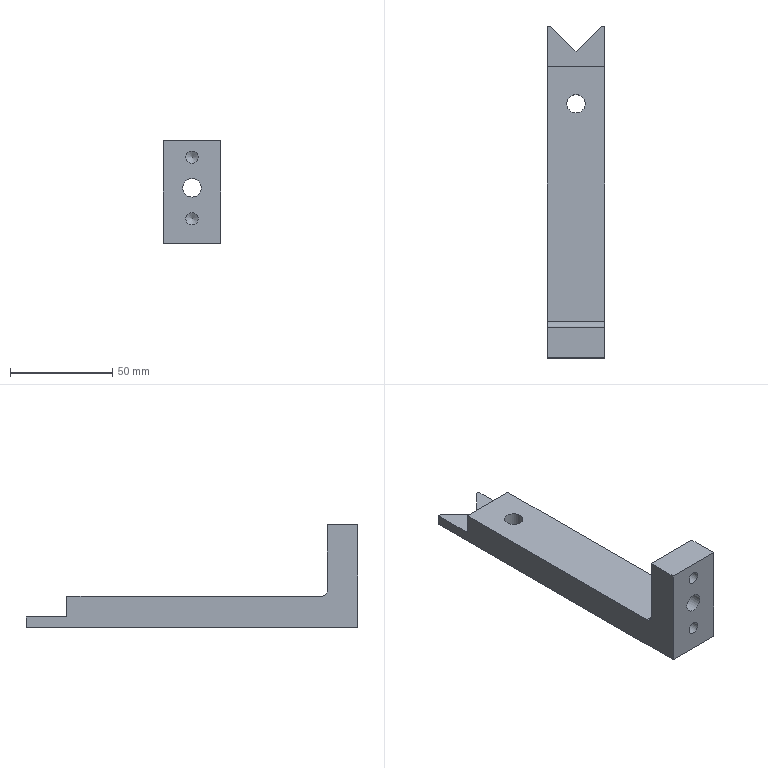Part | NX | features BREP 1 | 1 solid | 24 faces | box 28 x 162 x 50 mm | volume 73613 mm3 | plane 13 | cylinder 7 | cone 4 | commonest cylinder face diameters 6 x3 3.3 x2 9 x2
STEP:
#1=CARTESIAN_POINT('',(-4.5,43.,7.5));
#2=VERTEX_POINT('',#1);
#3=CARTESIAN_POINT('',(0.,43.,7.5));
#4=DIRECTION('',(0.,0.,-1.));
#5=DIRECTION('',(-1.,0.,0.));
#6=AXIS2_PLACEMENT_3D('',#3,#4,#5);
#7=CIRCLE('',#6,4.5);
#8=EDGE_CURVE('',#2,#2,#7,.T.);
#9=ORIENTED_EDGE('',*,*,#8,.T.);
#10=EDGE_LOOP('',(#9));
#11=FACE_BOUND('',#10,.T.);
#12=CARTESIAN_POINT('',(-14.,61.,7.5));
#13=VERTEX_POINT('',#12);
#14=CARTESIAN_POINT('',(-14.,-63.,7.5));
#15=VERTEX_POINT('',#14);
#16=CARTESIAN_POINT('',(-14.,-81.,7.5));
#17=DIRECTION('',(0.,-1.,0.));
#18=VECTOR('',#17,1000.);
#19=LINE('',#16,#18);
#20=EDGE_CURVE('',#13,#15,#19,.T.);
#21=ORIENTED_EDGE('',*,*,#20,.T.);
#22=CARTESIAN_POINT('',(14.,-63.,7.5));
#23=VERTEX_POINT('',#22);
#24=CARTESIAN_POINT('',(0.,-63.,7.5));
#25=DIRECTION('',(1.,0.,0.));
#26=VECTOR('',#25,1000.);
#27=LINE('',#24,#26);
#28=EDGE_CURVE('',#15,#23,#27,.T.);
#29=ORIENTED_EDGE('',*,*,#28,.T.);
#30=CARTESIAN_POINT('',(14.,61.,7.5));
#31=VERTEX_POINT('',#30);
#32=CARTESIAN_POINT('',(14.,-81.,7.5));
#33=DIRECTION('',(0.,1.,0.));
#34=VECTOR('',#33,1000.);
#35=LINE('',#32,#34);
#36=EDGE_CURVE('',#23,#31,#35,.T.);
#37=ORIENTED_EDGE('',*,*,#36,.T.);
#38=CARTESIAN_POINT('',(36.361,61.,7.5));
#39=DIRECTION('',(-1.,0.,0.));
#40=VECTOR('',#39,1000.);
#41=LINE('',#38,#40);
#42=EDGE_CURVE('',#31,#13,#41,.T.);
#43=ORIENTED_EDGE('',*,*,#42,.T.);
#44=EDGE_LOOP('',(#21,#29,#37,#43));
#45=FACE_BOUND('',#44,.T.);
#46=CARTESIAN_POINT('',(0.,0.,7.5));
#47=DIRECTION('',(0.,0.,-1.));
#48=DIRECTION('',(1.,0.,0.));
#49=AXIS2_PLACEMENT_3D('',#46,#47,#48);
#50=PLANE('',#49);
#51=ADVANCED_FACE('',(#11,#45),#50,.F.);
#52=CARTESIAN_POINT('',(-14.,81.,-2.5));
#53=VERTEX_POINT('',#52);
#54=CARTESIAN_POINT('',(-14.,81.,-7.5));
#55=VERTEX_POINT('',#54);
#56=CARTESIAN_POINT('',(-14.,81.,7.5));
#57=DIRECTION('',(0.,0.,-1.));
#58=VECTOR('',#57,1000.);
#59=LINE('',#56,#58);
#60=EDGE_CURVE('',#53,#55,#59,.T.);
#61=ORIENTED_EDGE('',*,*,#60,.F.);
#62=CARTESIAN_POINT('',(-12.5,81.,-2.5));
#63=VERTEX_POINT('',#62);
#64=CARTESIAN_POINT('',(36.361,81.,-2.5));
#65=DIRECTION('',(-1.,0.,0.));
#66=VECTOR('',#65,1000.);
#67=LINE('',#64,#66);
#68=EDGE_CURVE('',#63,#53,#67,.T.);
#69=ORIENTED_EDGE('',*,*,#68,.F.);
#70=CARTESIAN_POINT('',(-12.5,81.,-7.5));
#71=VERTEX_POINT('',#70);
#72=CARTESIAN_POINT('',(-12.5,81.,35.451));
#73=DIRECTION('',(0.,0.,-1.));
#74=VECTOR('',#73,1000.);
#75=LINE('',#72,#74);
#76=EDGE_CURVE('',#63,#71,#75,.T.);
#77=ORIENTED_EDGE('',*,*,#76,.T.);
#78=CARTESIAN_POINT('',(-14.,81.,-7.5));
#79=DIRECTION('',(-1.,0.,0.));
#80=VECTOR('',#79,1000.);
#81=LINE('',#78,#80);
#82=EDGE_CURVE('',#71,#55,#81,.T.);
#83=ORIENTED_EDGE('',*,*,#82,.T.);
#84=EDGE_LOOP('',(#61,#69,#77,#83));
#85=FACE_BOUND('',#84,.T.);
#86=CARTESIAN_POINT('',(-14.,81.,7.5));
#87=DIRECTION('',(0.,-1.,0.));
#88=DIRECTION('',(0.,0.,1.));
#89=AXIS2_PLACEMENT_3D('',#86,#87,#88);
#90=PLANE('',#89);
#91=ADVANCED_FACE('',(#85),#90,.F.);
#92=CARTESIAN_POINT('',(14.,61.,-2.5));
#93=VERTEX_POINT('',#92);
#94=CARTESIAN_POINT('',(14.,81.,-2.5));
#95=VERTEX_POINT('',#94);
#96=CARTESIAN_POINT('',(14.,61.,-2.5));
#97=DIRECTION('',(0.,1.,0.));
#98=VECTOR('',#97,1000.);
#99=LINE('',#96,#98);
#100=EDGE_CURVE('',#93,#95,#99,.T.);
#101=ORIENTED_EDGE('',*,*,#100,.F.);
#102=CARTESIAN_POINT('',(14.,61.,7.5));
#103=DIRECTION('',(0.,0.,-1.));
#104=VECTOR('',#103,1000.);
#105=LINE('',#102,#104);
#106=EDGE_CURVE('',#31,#93,#105,.T.);
#107=ORIENTED_EDGE('',*,*,#106,.F.);
#108=ORIENTED_EDGE('',*,*,#36,.F.);
#109=CARTESIAN_POINT('',(14.,-66.,10.5));
#110=VERTEX_POINT('',#109);
#111=CARTESIAN_POINT('',(14.,-63.,10.5));
#112=DIRECTION('',(-1.,0.,0.));
#113=DIRECTION('',(0.,0.,1.));
#114=AXIS2_PLACEMENT_3D('',#111,#112,#113);
#115=CIRCLE('',#114,3.);
#116=EDGE_CURVE('',#23,#110,#115,.T.);
#117=ORIENTED_EDGE('',*,*,#116,.T.);
#118=CARTESIAN_POINT('',(14.,-66.,42.5));
#119=VERTEX_POINT('',#118);
#120=CARTESIAN_POINT('',(14.,-66.,7.5));
#121=DIRECTION('',(0.,0.,1.));
#122=VECTOR('',#121,1000.);
#123=LINE('',#120,#122);
#124=EDGE_CURVE('',#110,#119,#123,.T.);
#125=ORIENTED_EDGE('',*,*,#124,.T.);
#126=CARTESIAN_POINT('',(14.,-81.,42.5));
#127=VERTEX_POINT('',#126);
#128=CARTESIAN_POINT('',(14.,-81.,42.5));
#129=DIRECTION('',(0.,-1.,0.));
#130=VECTOR('',#129,1000.);
#131=LINE('',#128,#130);
#132=EDGE_CURVE('',#119,#127,#131,.T.);
#133=ORIENTED_EDGE('',*,*,#132,.T.);
#134=CARTESIAN_POINT('',(14.,-81.,-7.5));
#135=VERTEX_POINT('',#134);
#136=CARTESIAN_POINT('',(14.,-81.,7.5));
#137=DIRECTION('',(0.,0.,-1.));
#138=VECTOR('',#137,1000.);
#139=LINE('',#136,#138);
#140=EDGE_CURVE('',#127,#135,#139,.T.);
#141=ORIENTED_EDGE('',*,*,#140,.T.);
#142=CARTESIAN_POINT('',(14.,81.,-7.5));
#143=VERTEX_POINT('',#142);
#144=CARTESIAN_POINT('',(14.,-81.,-7.5));
#145=DIRECTION('',(0.,1.,0.));
#146=VECTOR('',#145,1000.);
#147=LINE('',#144,#146);
#148=EDGE_CURVE('',#135,#143,#147,.T.);
#149=ORIENTED_EDGE('',*,*,#148,.T.);
#150=CARTESIAN_POINT('',(14.,81.,7.5));
#151=DIRECTION('',(0.,0.,-1.));
#152=VECTOR('',#151,1000.);
#153=LINE('',#150,#152);
#154=EDGE_CURVE('',#95,#143,#153,.T.);
#155=ORIENTED_EDGE('',*,*,#154,.F.);
#156=EDGE_LOOP('',(#101,#107,#108,#117,#125,#133,#141,#149,#155));
#157=FACE_BOUND('',#156,.T.);
#158=CARTESIAN_POINT('',(14.,-81.,7.5));
#159=DIRECTION('',(-1.,0.,0.));
#160=DIRECTION('',(0.,0.,-1.));
#161=AXIS2_PLACEMENT_3D('',#158,#159,#160);
#162=PLANE('',#161);
#163=ADVANCED_FACE('',(#157),#162,.F.);
#164=CARTESIAN_POINT('',(12.5,81.,-2.5));
#165=VERTEX_POINT('',#164);
#166=CARTESIAN_POINT('',(12.5,81.,-7.5));
#167=VERTEX_POINT('',#166);
#168=CARTESIAN_POINT('',(12.5,81.,35.451));
#169=DIRECTION('',(0.,0.,-1.));
#170=VECTOR('',#169,1000.);
#171=LINE('',#168,#170);
#172=EDGE_CURVE('',#165,#167,#171,.T.);
#173=ORIENTED_EDGE('',*,*,#172,.F.);
#174=CARTESIAN_POINT('',(36.361,81.,-2.5));
#175=DIRECTION('',(-1.,0.,0.));
#176=VECTOR('',#175,1000.);
#177=LINE('',#174,#176);
#178=EDGE_CURVE('',#95,#165,#177,.T.);
#179=ORIENTED_EDGE('',*,*,#178,.F.);
#180=ORIENTED_EDGE('',*,*,#154,.T.);
#181=CARTESIAN_POINT('',(-14.,81.,-7.5));
#182=DIRECTION('',(-1.,0.,0.));
#183=VECTOR('',#182,1000.);
#184=LINE('',#181,#183);
#185=EDGE_CURVE('',#143,#167,#184,.T.);
#186=ORIENTED_EDGE('',*,*,#185,.T.);
#187=EDGE_LOOP('',(#173,#179,#180,#186));
#188=FACE_BOUND('',#187,.T.);
#189=CARTESIAN_POINT('',(-14.,81.,7.5));
#190=DIRECTION('',(0.,-1.,0.));
#191=DIRECTION('',(0.,0.,1.));
#192=AXIS2_PLACEMENT_3D('',#189,#190,#191);
#193=PLANE('',#192);
#194=ADVANCED_FACE('',(#188),#193,.F.);
#195=ORIENTED_EDGE('',*,*,#20,.F.);
#196=CARTESIAN_POINT('',(-14.,61.,-2.5));
#197=VERTEX_POINT('',#196);
#198=CARTESIAN_POINT('',(-14.,61.,7.5));
#199=DIRECTION('',(0.,0.,1.));
#200=VECTOR('',#199,1000.);
#201=LINE('',#198,#200);
#202=EDGE_CURVE('',#197,#13,#201,.T.);
#203=ORIENTED_EDGE('',*,*,#202,.F.);
#204=CARTESIAN_POINT('',(-14.,61.,-2.5));
#205=DIRECTION('',(0.,-1.,0.));
#206=VECTOR('',#205,1000.);
#207=LINE('',#204,#206);
#208=EDGE_CURVE('',#53,#197,#207,.T.);
#209=ORIENTED_EDGE('',*,*,#208,.F.);
#210=ORIENTED_EDGE('',*,*,#60,.T.);
#211=CARTESIAN_POINT('',(-14.,-81.,-7.5));
#212=VERTEX_POINT('',#211);
#213=CARTESIAN_POINT('',(-14.,-81.,-7.5));
#214=DIRECTION('',(0.,-1.,0.));
#215=VECTOR('',#214,1000.);
#216=LINE('',#213,#215);
#217=EDGE_CURVE('',#55,#212,#216,.T.);
#218=ORIENTED_EDGE('',*,*,#217,.T.);
#219=CARTESIAN_POINT('',(-14.,-81.,42.5));
#220=VERTEX_POINT('',#219);
#221=CARTESIAN_POINT('',(-14.,-81.,7.5));
#222=DIRECTION('',(0.,0.,-1.));
#223=VECTOR('',#222,1000.);
#224=LINE('',#221,#223);
#225=EDGE_CURVE('',#220,#212,#224,.T.);
#226=ORIENTED_EDGE('',*,*,#225,.F.);
#227=CARTESIAN_POINT('',(-14.,-66.,42.5));
#228=VERTEX_POINT('',#227);
#229=CARTESIAN_POINT('',(-14.,-81.,42.5));
#230=DIRECTION('',(0.,1.,0.));
#231=VECTOR('',#230,1000.);
#232=LINE('',#229,#231);
#233=EDGE_CURVE('',#220,#228,#232,.T.);
#234=ORIENTED_EDGE('',*,*,#233,.T.);
#235=CARTESIAN_POINT('',(-14.,-66.,10.5));
#236=VERTEX_POINT('',#235);
#237=CARTESIAN_POINT('',(-14.,-66.,7.5));
#238=DIRECTION('',(0.,0.,-1.));
#239=VECTOR('',#238,1000.);
#240=LINE('',#237,#239);
#241=EDGE_CURVE('',#228,#236,#240,.T.);
#242=ORIENTED_EDGE('',*,*,#241,.T.);
#243=CARTESIAN_POINT('',(-14.,-63.,10.5));
#244=DIRECTION('',(1.,0.,0.));
#245=DIRECTION('',(0.,0.,-1.));
#246=AXIS2_PLACEMENT_3D('',#243,#244,#245);
#247=CIRCLE('',#246,3.);
#248=EDGE_CURVE('',#236,#15,#247,.T.);
#249=ORIENTED_EDGE('',*,*,#248,.T.);
#250=EDGE_LOOP('',(#195,#203,#209,#210,#218,#226,#234,#242,#249));
#251=FACE_BOUND('',#250,.T.);
#252=CARTESIAN_POINT('',(-14.,-81.,7.5));
#253=DIRECTION('',(1.,0.,0.));
#254=DIRECTION('',(0.,0.,1.));
#255=AXIS2_PLACEMENT_3D('',#252,#253,#254);
#256=PLANE('',#255);
#257=ADVANCED_FACE('',(#251),#256,.F.);
#258=CARTESIAN_POINT('',(0.,-81.,24.));
#259=VERTEX_POINT('',#258);
#260=CARTESIAN_POINT('',(0.,-81.,19.5));
#261=DIRECTION('',(0.,1.,0.));
#262=DIRECTION('',(0.,0.,1.));
#263=AXIS2_PLACEMENT_3D('',#260,#261,#262);
#264=CIRCLE('',#263,4.5);
#265=EDGE_CURVE('',#259,#259,#264,.T.);
#266=ORIENTED_EDGE('',*,*,#265,.T.);
#267=EDGE_LOOP('',(#266));
#268=FACE_BOUND('',#267,.T.);
#269=CARTESIAN_POINT('',(0.,-81.,31.5));
#270=VERTEX_POINT('',#269);
#271=CARTESIAN_POINT('',(0.,-81.,34.5));
#272=DIRECTION('',(0.,-1.,0.));
#273=DIRECTION('',(0.,0.,-1.));
#274=AXIS2_PLACEMENT_3D('',#271,#272,#273);
#275=CIRCLE('',#274,3.);
#276=EDGE_CURVE('',#270,#270,#275,.T.);
#277=ORIENTED_EDGE('',*,*,#276,.F.);
#278=EDGE_LOOP('',(#277));
#279=FACE_BOUND('',#278,.T.);
#280=CARTESIAN_POINT('',(0.,-81.,1.5));
#281=VERTEX_POINT('',#280);
#282=CARTESIAN_POINT('',(0.,-81.,4.5));
#283=DIRECTION('',(0.,-1.,0.));
#284=DIRECTION('',(0.,0.,-1.));
#285=AXIS2_PLACEMENT_3D('',#282,#283,#284);
#286=CIRCLE('',#285,3.);
#287=EDGE_CURVE('',#281,#281,#286,.T.);
#288=ORIENTED_EDGE('',*,*,#287,.F.);
#289=EDGE_LOOP('',(#288));
#290=FACE_BOUND('',#289,.T.);
#291=CARTESIAN_POINT('',(-14.,-81.,-7.5));
#292=DIRECTION('',(1.,0.,0.));
#293=VECTOR('',#292,1000.);
#294=LINE('',#291,#293);
#295=EDGE_CURVE('',#212,#135,#294,.T.);
#296=ORIENTED_EDGE('',*,*,#295,.T.);
#297=ORIENTED_EDGE('',*,*,#140,.F.);
#298=CARTESIAN_POINT('',(52.079,-81.,42.5));
#299=DIRECTION('',(-1.,0.,0.));
#300=VECTOR('',#299,1000.);
#301=LINE('',#298,#300);
#302=EDGE_CURVE('',#127,#220,#301,.T.);
#303=ORIENTED_EDGE('',*,*,#302,.T.);
#304=ORIENTED_EDGE('',*,*,#225,.T.);
#305=EDGE_LOOP('',(#296,#297,#303,#304));
#306=FACE_BOUND('',#305,.T.);
#307=CARTESIAN_POINT('',(-14.,-81.,7.5));
#308=DIRECTION('',(0.,1.,0.));
#309=DIRECTION('',(0.,0.,-1.));
#310=AXIS2_PLACEMENT_3D('',#307,#308,#309);
#311=PLANE('',#310);
#312=ADVANCED_FACE('',(#268,#279,#290,#306),#311,.F.);
#313=CARTESIAN_POINT('',(8.35,36.881,-7.5));
#314=VERTEX_POINT('',#313);
#315=CARTESIAN_POINT('',(10.,36.881,-7.5));
#316=DIRECTION('',(0.,0.,-1.));
#317=DIRECTION('',(-1.,0.,0.));
#318=AXIS2_PLACEMENT_3D('',#315,#316,#317);
#319=CIRCLE('',#318,1.65);
#320=EDGE_CURVE('',#314,#314,#319,.T.);
#321=ORIENTED_EDGE('',*,*,#320,.F.);
#322=EDGE_LOOP('',(#321));
#323=FACE_BOUND('',#322,.T.);
#324=CARTESIAN_POINT('',(-11.65,36.881,-7.5));
#325=VERTEX_POINT('',#324);
#326=CARTESIAN_POINT('',(-10.,36.881,-7.5));
#327=DIRECTION('',(0.,0.,-1.));
#328=DIRECTION('',(-1.,0.,0.));
#329=AXIS2_PLACEMENT_3D('',#326,#327,#328);
#330=CIRCLE('',#329,1.65);
#331=EDGE_CURVE('',#325,#325,#330,.T.);
#332=ORIENTED_EDGE('',*,*,#331,.F.);
#333=EDGE_LOOP('',(#332));
#334=FACE_BOUND('',#333,.T.);
#335=CARTESIAN_POINT('',(-4.5,43.,-7.5));
#336=VERTEX_POINT('',#335);
#337=CARTESIAN_POINT('',(0.,43.,-7.5));
#338=DIRECTION('',(0.,0.,-1.));
#339=DIRECTION('',(-1.,0.,0.));
#340=AXIS2_PLACEMENT_3D('',#337,#338,#339);
#341=CIRCLE('',#340,4.5);
#342=EDGE_CURVE('',#336,#336,#341,.T.);
#343=ORIENTED_EDGE('',*,*,#342,.F.);
#344=EDGE_LOOP('',(#343));
#345=FACE_BOUND('',#344,.T.);
#346=CARTESIAN_POINT('',(0.,68.5,-7.5));
#347=VERTEX_POINT('',#346);
#348=CARTESIAN_POINT('',(0.,68.5,-7.5));
#349=DIRECTION('',(-0.7071,0.7071,0.));
#350=VECTOR('',#349,1000.);
#351=LINE('',#348,#350);
#352=EDGE_CURVE('',#347,#71,#351,.T.);
#353=ORIENTED_EDGE('',*,*,#352,.F.);
#354=CARTESIAN_POINT('',(12.5,81.,-7.5));
#355=DIRECTION('',(-0.7071,-0.7071,0.));
#356=VECTOR('',#355,1000.);
#357=LINE('',#354,#356);
#358=EDGE_CURVE('',#167,#347,#357,.T.);
#359=ORIENTED_EDGE('',*,*,#358,.F.);
#360=ORIENTED_EDGE('',*,*,#185,.F.);
#361=ORIENTED_EDGE('',*,*,#148,.F.);
#362=ORIENTED_EDGE('',*,*,#295,.F.);
#363=ORIENTED_EDGE('',*,*,#217,.F.);
#364=ORIENTED_EDGE('',*,*,#82,.F.);
#365=EDGE_LOOP('',(#353,#359,#360,#361,#362,#363,#364));
#366=FACE_BOUND('',#365,.T.);
#367=CARTESIAN_POINT('',(0.,0.,-7.5));
#368=DIRECTION('',(0.,0.,-1.));
#369=DIRECTION('',(1.,0.,0.));
#370=AXIS2_PLACEMENT_3D('',#367,#368,#369);
#371=PLANE('',#370);
#372=ADVANCED_FACE('',(#323,#334,#345,#366),#371,.T.);
#373=ORIENTED_EDGE('',*,*,#76,.F.);
#374=CARTESIAN_POINT('',(0.,68.5,-2.5));
#375=VERTEX_POINT('',#374);
#376=CARTESIAN_POINT('',(0.,68.5,-2.5));
#377=DIRECTION('',(0.7071,-0.7071,0.));
#378=VECTOR('',#377,1000.);
#379=LINE('',#376,#378);
#380=EDGE_CURVE('',#63,#375,#379,.T.);
#381=ORIENTED_EDGE('',*,*,#380,.T.);
#382=CARTESIAN_POINT('',(0.,68.5,35.451));
#383=DIRECTION('',(0.,0.,-1.));
#384=VECTOR('',#383,1000.);
#385=LINE('',#382,#384);
#386=EDGE_CURVE('',#375,#347,#385,.T.);
#387=ORIENTED_EDGE('',*,*,#386,.T.);
#388=ORIENTED_EDGE('',*,*,#352,.T.);
#389=EDGE_LOOP('',(#373,#381,#387,#388));
#390=FACE_BOUND('',#389,.T.);
#391=CARTESIAN_POINT('',(0.,68.5,35.451));
#392=DIRECTION('',(-0.7071,-0.7071,0.));
#393=DIRECTION('',(-0.7071,0.7071,0.));
#394=AXIS2_PLACEMENT_3D('',#391,#392,#393);
#395=PLANE('',#394);
#396=ADVANCED_FACE('',(#390),#395,.F.);
#397=ORIENTED_EDGE('',*,*,#386,.F.);
#398=CARTESIAN_POINT('',(12.5,81.,-2.5));
#399=DIRECTION('',(0.7071,0.7071,0.));
#400=VECTOR('',#399,1000.);
#401=LINE('',#398,#400);
#402=EDGE_CURVE('',#375,#165,#401,.T.);
#403=ORIENTED_EDGE('',*,*,#402,.T.);
#404=ORIENTED_EDGE('',*,*,#172,.T.);
#405=ORIENTED_EDGE('',*,*,#358,.T.);
#406=EDGE_LOOP('',(#397,#403,#404,#405));
#407=FACE_BOUND('',#406,.T.);
#408=CARTESIAN_POINT('',(12.5,81.,35.451));
#409=DIRECTION('',(0.7071,-0.7071,0.));
#410=DIRECTION('',(-0.7071,-0.7071,0.));
#411=AXIS2_PLACEMENT_3D('',#408,#409,#410);
#412=PLANE('',#411);
#413=ADVANCED_FACE('',(#407),#412,.F.);
#414=ORIENTED_EDGE('',*,*,#68,.T.);
#415=ORIENTED_EDGE('',*,*,#208,.T.);
#416=CARTESIAN_POINT('',(36.361,61.,-2.5));
#417=DIRECTION('',(-1.,0.,0.));
#418=VECTOR('',#417,1000.);
#419=LINE('',#416,#418);
#420=EDGE_CURVE('',#93,#197,#419,.T.);
#421=ORIENTED_EDGE('',*,*,#420,.F.);
#422=ORIENTED_EDGE('',*,*,#100,.T.);
#423=ORIENTED_EDGE('',*,*,#178,.T.);
#424=ORIENTED_EDGE('',*,*,#402,.F.);
#425=ORIENTED_EDGE('',*,*,#380,.F.);
#426=EDGE_LOOP('',(#414,#415,#421,#422,#423,#424,#425));
#427=FACE_BOUND('',#426,.T.);
#428=CARTESIAN_POINT('',(36.361,61.,-2.5));
#429=DIRECTION('',(0.,0.,-1.));
#430=DIRECTION('',(0.,-1.,0.));
#431=AXIS2_PLACEMENT_3D('',#428,#429,#430);
#432=PLANE('',#431);
#433=ADVANCED_FACE('',(#427),#432,.F.);
#434=ORIENTED_EDGE('',*,*,#106,.T.);
#435=ORIENTED_EDGE('',*,*,#420,.T.);
#436=ORIENTED_EDGE('',*,*,#202,.T.);
#437=ORIENTED_EDGE('',*,*,#42,.F.);
#438=EDGE_LOOP('',(#434,#435,#436,#437));
#439=FACE_BOUND('',#438,.T.);
#440=CARTESIAN_POINT('',(36.361,61.,7.5));
#441=DIRECTION('',(0.,-1.,0.));
#442=DIRECTION('',(0.,0.,1.));
#443=AXIS2_PLACEMENT_3D('',#440,#441,#442);
#444=PLANE('',#443);
#445=ADVANCED_FACE('',(#439),#444,.F.);
#446=CARTESIAN_POINT('',(0.,-66.,24.));
#447=VERTEX_POINT('',#446);
#448=CARTESIAN_POINT('',(0.,-66.,19.5));
#449=DIRECTION('',(0.,1.,0.));
#450=DIRECTION('',(0.,0.,1.));
#451=AXIS2_PLACEMENT_3D('',#448,#449,#450);
#452=CIRCLE('',#451,4.5);
#453=EDGE_CURVE('',#447,#447,#452,.T.);
#454=ORIENTED_EDGE('',*,*,#453,.F.);
#455=EDGE_LOOP('',(#454));
#456=FACE_BOUND('',#455,.T.);
#457=ORIENTED_EDGE('',*,*,#124,.F.);
#458=CARTESIAN_POINT('',(52.079,-66.,10.5));
#459=DIRECTION('',(-1.,0.,0.));
#460=VECTOR('',#459,1000.);
#461=LINE('',#458,#460);
#462=EDGE_CURVE('',#110,#236,#461,.T.);
#463=ORIENTED_EDGE('',*,*,#462,.T.);
#464=ORIENTED_EDGE('',*,*,#241,.F.);
#465=CARTESIAN_POINT('',(52.079,-66.,42.5));
#466=DIRECTION('',(-1.,0.,0.));
#467=VECTOR('',#466,1000.);
#468=LINE('',#465,#467);
#469=EDGE_CURVE('',#119,#228,#468,.T.);
#470=ORIENTED_EDGE('',*,*,#469,.F.);
#471=EDGE_LOOP('',(#457,#463,#464,#470));
#472=FACE_BOUND('',#471,.T.);
#473=CARTESIAN_POINT('',(52.079,-66.,7.5));
#474=DIRECTION('',(0.,1.,0.));
#475=DIRECTION('',(0.,0.,-1.));
#476=AXIS2_PLACEMENT_3D('',#473,#474,#475);
#477=PLANE('',#476);
#478=ADVANCED_FACE('',(#456,#472),#477,.T.);
#479=ORIENTED_EDGE('',*,*,#132,.F.);
#480=ORIENTED_EDGE('',*,*,#469,.T.);
#481=ORIENTED_EDGE('',*,*,#233,.F.);
#482=ORIENTED_EDGE('',*,*,#302,.F.);
#483=EDGE_LOOP('',(#479,#480,#481,#482));
#484=FACE_BOUND('',#483,.T.);
#485=CARTESIAN_POINT('',(52.079,-81.,42.5));
#486=DIRECTION('',(0.,0.,1.));
#487=DIRECTION('',(-1.,0.,0.));
#488=AXIS2_PLACEMENT_3D('',#485,#486,#487);
#489=PLANE('',#488);
#490=ADVANCED_FACE('',(#484),#489,.T.);
#491=CARTESIAN_POINT('',(0.,-67.197,4.5));
#492=VERTEX_POINT('',#491);
#493=VERTEX_LOOP('',#492);
#494=FACE_BOUND('',#493,.T.);
#495=CARTESIAN_POINT('',(0.,-69.,1.5));
#496=VERTEX_POINT('',#495);
#497=CARTESIAN_POINT('',(0.,-69.,4.5));
#498=DIRECTION('',(0.,-1.,0.));
#499=DIRECTION('',(0.,0.,-1.));
#500=AXIS2_PLACEMENT_3D('',#497,#498,#499);
#501=CIRCLE('',#500,3.);
#502=EDGE_CURVE('',#496,#496,#501,.T.);
#503=ORIENTED_EDGE('',*,*,#502,.T.);
#504=EDGE_LOOP('',(#503));
#505=FACE_BOUND('',#504,.T.);
#506=CARTESIAN_POINT('',(0.,-69.,4.5));
#507=DIRECTION('',(0.,-1.,0.));
#508=DIRECTION('',(0.,0.,1.));
#509=AXIS2_PLACEMENT_3D('',#506,#507,#508);
#510=CONICAL_SURFACE('',#509,3.,1.03);
#511=ADVANCED_FACE('',(#494,#505),#510,.F.);
#512=ORIENTED_EDGE('',*,*,#502,.F.);
#513=EDGE_LOOP('',(#512));
#514=FACE_BOUND('',#513,.T.);
#515=ORIENTED_EDGE('',*,*,#287,.T.);
#516=EDGE_LOOP('',(#515));
#517=FACE_BOUND('',#516,.T.);
#518=CARTESIAN_POINT('',(0.,-81.,4.5));
#519=DIRECTION('',(0.,-1.,0.));
#520=DIRECTION('',(0.,0.,1.));
#521=AXIS2_PLACEMENT_3D('',#518,#519,#520);
#522=CYLINDRICAL_SURFACE('',#521,3.);
#523=ADVANCED_FACE('',(#514,#517),#522,.F.);
#524=CARTESIAN_POINT('',(0.,-67.197,34.5));
#525=VERTEX_POINT('',#524);
#526=VERTEX_LOOP('',#525);
#527=FACE_BOUND('',#526,.T.);
#528=CARTESIAN_POINT('',(0.,-69.,31.5));
#529=VERTEX_POINT('',#528);
#530=CARTESIAN_POINT('',(0.,-69.,34.5));
#531=DIRECTION('',(0.,-1.,0.));
#532=DIRECTION('',(0.,0.,-1.));
#533=AXIS2_PLACEMENT_3D('',#530,#531,#532);
#534=CIRCLE('',#533,3.);
#535=EDGE_CURVE('',#529,#529,#534,.T.);
#536=ORIENTED_EDGE('',*,*,#535,.T.);
#537=EDGE_LOOP('',(#536));
#538=FACE_BOUND('',#537,.T.);
#539=CARTESIAN_POINT('',(0.,-69.,34.5));
#540=DIRECTION('',(0.,-1.,0.));
#541=DIRECTION('',(0.,0.,1.));
#542=AXIS2_PLACEMENT_3D('',#539,#540,#541);
#543=CONICAL_SURFACE('',#542,3.,1.03);
#544=ADVANCED_FACE('',(#527,#538),#543,.F.);
#545=ORIENTED_EDGE('',*,*,#535,.F.);
#546=EDGE_LOOP('',(#545));
#547=FACE_BOUND('',#546,.T.);
#548=ORIENTED_EDGE('',*,*,#276,.T.);
#549=EDGE_LOOP('',(#548));
#550=FACE_BOUND('',#549,.T.);
#551=CARTESIAN_POINT('',(0.,-81.,34.5));
#552=DIRECTION('',(0.,-1.,0.));
#553=DIRECTION('',(0.,0.,1.));
#554=AXIS2_PLACEMENT_3D('',#551,#552,#553);
#555=CYLINDRICAL_SURFACE('',#554,3.);
#556=ADVANCED_FACE('',(#547,#550),#555,.F.);
#557=ORIENTED_EDGE('',*,*,#265,.F.);
#558=EDGE_LOOP('',(#557));
#559=FACE_BOUND('',#558,.T.);
#560=ORIENTED_EDGE('',*,*,#453,.T.);
#561=EDGE_LOOP('',(#560));
#562=FACE_BOUND('',#561,.T.);
#563=CARTESIAN_POINT('',(0.,-66.,19.5));
#564=DIRECTION('',(0.,1.,0.));
#565=DIRECTION('',(0.,0.,-1.));
#566=AXIS2_PLACEMENT_3D('',#563,#564,#565);
#567=CYLINDRICAL_SURFACE('',#566,4.5);
#568=ADVANCED_FACE('',(#559,#562),#567,.F.);
#569=ORIENTED_EDGE('',*,*,#116,.F.);
#570=ORIENTED_EDGE('',*,*,#28,.F.);
#571=ORIENTED_EDGE('',*,*,#248,.F.);
#572=ORIENTED_EDGE('',*,*,#462,.F.);
#573=EDGE_LOOP('',(#569,#570,#571,#572));
#574=FACE_BOUND('',#573,.T.);
#575=CARTESIAN_POINT('',(52.079,-63.,10.5));
#576=DIRECTION('',(-1.,0.,0.));
#577=DIRECTION('',(0.,0.,-1.));
#578=AXIS2_PLACEMENT_3D('',#575,#576,#577);
#579=CYLINDRICAL_SURFACE('',#578,3.);
#580=ADVANCED_FACE('',(#574),#579,.F.);
#581=ORIENTED_EDGE('',*,*,#342,.T.);
#582=EDGE_LOOP('',(#581));
#583=FACE_BOUND('',#582,.T.);
#584=ORIENTED_EDGE('',*,*,#8,.F.);
#585=EDGE_LOOP('',(#584));
#586=FACE_BOUND('',#585,.T.);
#587=CARTESIAN_POINT('',(0.,43.,-7.5));
#588=DIRECTION('',(0.,0.,-1.));
#589=DIRECTION('',(1.,0.,0.));
#590=AXIS2_PLACEMENT_3D('',#587,#588,#589);
#591=CYLINDRICAL_SURFACE('',#590,4.5);
#592=ADVANCED_FACE('',(#583,#586),#591,.F.);
#593=CARTESIAN_POINT('',(-10.,36.881,3.591));
#594=VERTEX_POINT('',#593);
#595=VERTEX_LOOP('',#594);
#596=FACE_BOUND('',#595,.T.);
#597=CARTESIAN_POINT('',(-11.65,36.881,2.6));
#598=VERTEX_POINT('',#597);
#599=CARTESIAN_POINT('',(-10.,36.881,2.6));
#600=DIRECTION('',(0.,0.,-1.));
#601=DIRECTION('',(-1.,0.,0.));
#602=AXIS2_PLACEMENT_3D('',#599,#600,#601);
#603=CIRCLE('',#602,1.65);
#604=EDGE_CURVE('',#598,#598,#603,.T.);
#605=ORIENTED_EDGE('',*,*,#604,.T.);
#606=EDGE_LOOP('',(#605));
#607=FACE_BOUND('',#606,.T.);
#608=CARTESIAN_POINT('',(-10.,36.881,2.6));
#609=DIRECTION('',(0.,0.,-1.));
#610=DIRECTION('',(1.,0.,0.));
#611=AXIS2_PLACEMENT_3D('',#608,#609,#610);
#612=CONICAL_SURFACE('',#611,1.65,1.03);
#613=ADVANCED_FACE('',(#596,#607),#612,.F.);
#614=ORIENTED_EDGE('',*,*,#604,.F.);
#615=EDGE_LOOP('',(#614));
#616=FACE_BOUND('',#615,.T.);
#617=ORIENTED_EDGE('',*,*,#331,.T.);
#618=EDGE_LOOP('',(#617));
#619=FACE_BOUND('',#618,.T.);
#620=CARTESIAN_POINT('',(-10.,36.881,-7.5));
#621=DIRECTION('',(0.,0.,-1.));
#622=DIRECTION('',(1.,0.,0.));
#623=AXIS2_PLACEMENT_3D('',#620,#621,#622);
#624=CYLINDRICAL_SURFACE('',#623,1.65);
#625=ADVANCED_FACE('',(#616,#619),#624,.F.);
#626=CARTESIAN_POINT('',(10.,36.881,3.591));
#627=VERTEX_POINT('',#626);
#628=VERTEX_LOOP('',#627);
#629=FACE_BOUND('',#628,.T.);
#630=CARTESIAN_POINT('',(8.35,36.881,2.6));
#631=VERTEX_POINT('',#630);
#632=CARTESIAN_POINT('',(10.,36.881,2.6));
#633=DIRECTION('',(0.,0.,-1.));
#634=DIRECTION('',(-1.,0.,0.));
#635=AXIS2_PLACEMENT_3D('',#632,#633,#634);
#636=CIRCLE('',#635,1.65);
#637=EDGE_CURVE('',#631,#631,#636,.T.);
#638=ORIENTED_EDGE('',*,*,#637,.T.);
#639=EDGE_LOOP('',(#638));
#640=FACE_BOUND('',#639,.T.);
#641=CARTESIAN_POINT('',(10.,36.881,2.6));
#642=DIRECTION('',(0.,0.,-1.));
#643=DIRECTION('',(1.,0.,0.));
#644=AXIS2_PLACEMENT_3D('',#641,#642,#643);
#645=CONICAL_SURFACE('',#644,1.65,1.03);
#646=ADVANCED_FACE('',(#629,#640),#645,.F.);
#647=ORIENTED_EDGE('',*,*,#637,.F.);
#648=EDGE_LOOP('',(#647));
#649=FACE_BOUND('',#648,.T.);
#650=ORIENTED_EDGE('',*,*,#320,.T.);
#651=EDGE_LOOP('',(#650));
#652=FACE_BOUND('',#651,.T.);
#653=CARTESIAN_POINT('',(10.,36.881,-7.5));
#654=DIRECTION('',(0.,0.,-1.));
#655=DIRECTION('',(1.,0.,0.));
#656=AXIS2_PLACEMENT_3D('',#653,#654,#655);
#657=CYLINDRICAL_SURFACE('',#656,1.65);
#658=ADVANCED_FACE('',(#649,#652),#657,.F.);
#659=CLOSED_SHELL('',(#51,#91,#163,#194,#257,#312,#372,#396,#413,#433,#445,#478,#490,#511,#523,#544,#556,#568,#580,#592,#613,#625,#646,#658));
#660=MANIFOLD_SOLID_BREP('',#659);
#661=(LENGTH_UNIT()NAMED_UNIT(*)SI_UNIT(.MILLI.,.METRE.));
#662=UNCERTAINTY_MEASURE_WITH_UNIT(LENGTH_MEASURE(0.00001),#661,'','');
#663=(NAMED_UNIT(*)PLANE_ANGLE_UNIT()SI_UNIT($,.RADIAN.));
#664=(NAMED_UNIT(*)SI_UNIT($,.STERADIAN.)SOLID_ANGLE_UNIT());
#665=(GEOMETRIC_REPRESENTATION_CONTEXT(3)GLOBAL_UNCERTAINTY_ASSIGNED_CONTEXT((#662))GLOBAL_UNIT_ASSIGNED_CONTEXT((#661,#663,#664))REPRESENTATION_CONTEXT('',''));
#666=ADVANCED_BREP_SHAPE_REPRESENTATION('',(#660),#665);